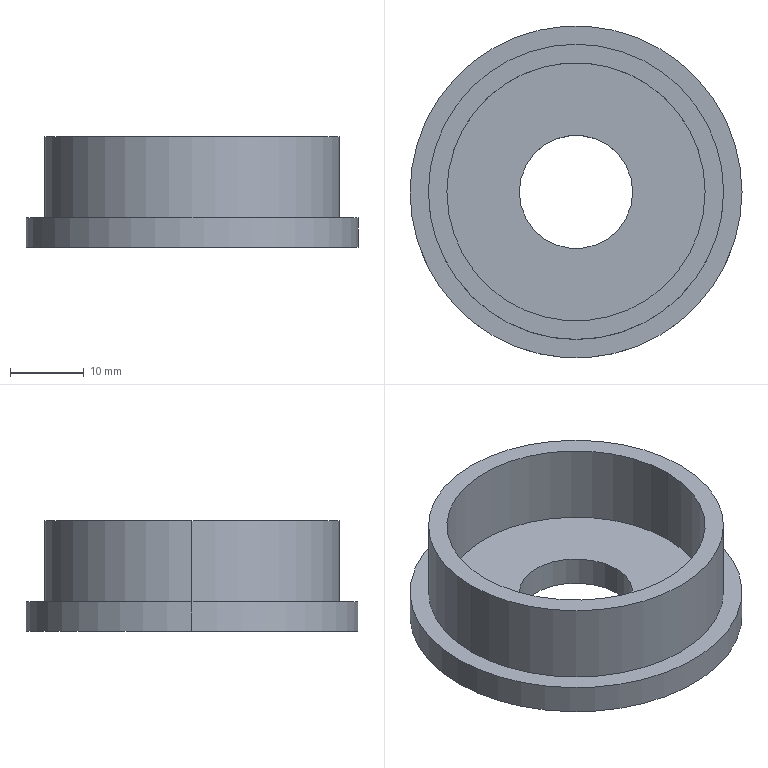Part | SolidWorks | features ICE 2, Extrusion 1 | 1 solid | 12 faces | box 45 x 45 x 15 mm | volume 8861 mm3 | cylinder 8 | plane 4 | commonest cylinder face diameters 15.357 x2 35 x2 40 x2 45 x2
STEP:
#1=CARTESIAN_POINT('',(-7.679,0.,-2.));
#2=VERTEX_POINT('',#1);
#3=CARTESIAN_POINT('',(7.679,0.,-2.));
#4=VERTEX_POINT('',#3);
#5=CARTESIAN_POINT('',(0.,0.,-2.));
#6=DIRECTION('',(0.,0.,1.));
#7=DIRECTION('',(1.,0.,0.));
#8=AXIS2_PLACEMENT_3D('',#5,#6,#7);
#9=CIRCLE('',#8,7.679);
#10=EDGE_CURVE('',#2,#4,#9,.T.);
#11=ORIENTED_EDGE('',*,*,#10,.F.);
#12=CARTESIAN_POINT('',(-7.679,0.,2.));
#13=VERTEX_POINT('',#12);
#14=CARTESIAN_POINT('',(-7.679,0.,-19.));
#15=DIRECTION('',(0.,0.,1.));
#16=VECTOR('',#15,1000.);
#17=LINE('',#14,#16);
#18=EDGE_CURVE('',#2,#13,#17,.T.);
#19=ORIENTED_EDGE('',*,*,#18,.T.);
#20=CARTESIAN_POINT('',(7.679,0.,2.));
#21=VERTEX_POINT('',#20);
#22=CARTESIAN_POINT('',(0.,0.,2.));
#23=DIRECTION('',(0.,0.,1.));
#24=DIRECTION('',(1.,0.,0.));
#25=AXIS2_PLACEMENT_3D('',#22,#23,#24);
#26=CIRCLE('',#25,7.679);
#27=EDGE_CURVE('',#13,#21,#26,.T.);
#28=ORIENTED_EDGE('',*,*,#27,.T.);
#29=CARTESIAN_POINT('',(7.679,0.,-19.));
#30=DIRECTION('',(0.,0.,1.));
#31=VECTOR('',#30,1000.);
#32=LINE('',#29,#31);
#33=EDGE_CURVE('',#4,#21,#32,.T.);
#34=ORIENTED_EDGE('',*,*,#33,.F.);
#35=EDGE_LOOP('',(#11,#19,#28,#34));
#36=FACE_OUTER_BOUND('',#35,.T.);
#37=CARTESIAN_POINT('',(0.,0.,-19.));
#38=DIRECTION('',(0.,0.,1.));
#39=DIRECTION('',(1.,0.,0.));
#40=AXIS2_PLACEMENT_3D('',#37,#38,#39);
#41=CYLINDRICAL_SURFACE('',#40,7.679);
#42=ADVANCED_FACE('',(#36),#41,.F.);
#43=CARTESIAN_POINT('',(-17.5,0.,13.));
#44=VERTEX_POINT('',#43);
#45=CARTESIAN_POINT('',(17.5,0.,13.));
#46=VERTEX_POINT('',#45);
#47=CARTESIAN_POINT('',(0.,0.,13.));
#48=DIRECTION('',(0.,0.,1.));
#49=DIRECTION('',(1.,0.,0.));
#50=AXIS2_PLACEMENT_3D('',#47,#48,#49);
#51=CIRCLE('',#50,17.5);
#52=EDGE_CURVE('',#44,#46,#51,.T.);
#53=ORIENTED_EDGE('',*,*,#52,.T.);
#54=CARTESIAN_POINT('',(17.5,0.,2.));
#55=VERTEX_POINT('',#54);
#56=CARTESIAN_POINT('',(17.5,0.,13.));
#57=DIRECTION('',(0.,0.,-1.));
#58=VECTOR('',#57,1000.);
#59=LINE('',#56,#58);
#60=EDGE_CURVE('',#46,#55,#59,.T.);
#61=ORIENTED_EDGE('',*,*,#60,.T.);
#62=CARTESIAN_POINT('',(-17.5,0.,2.));
#63=VERTEX_POINT('',#62);
#64=CARTESIAN_POINT('',(0.,0.,2.));
#65=DIRECTION('',(0.,0.,-1.));
#66=DIRECTION('',(1.,0.,0.));
#67=AXIS2_PLACEMENT_3D('',#64,#65,#66);
#68=CIRCLE('',#67,17.5);
#69=EDGE_CURVE('',#55,#63,#68,.T.);
#70=ORIENTED_EDGE('',*,*,#69,.T.);
#71=CARTESIAN_POINT('',(-17.5,0.,13.));
#72=DIRECTION('',(0.,0.,-1.));
#73=VECTOR('',#72,1000.);
#74=LINE('',#71,#73);
#75=EDGE_CURVE('',#44,#63,#74,.T.);
#76=ORIENTED_EDGE('',*,*,#75,.F.);
#77=EDGE_LOOP('',(#53,#61,#70,#76));
#78=FACE_OUTER_BOUND('',#77,.T.);
#79=CARTESIAN_POINT('',(0.,0.,13.));
#80=DIRECTION('',(0.,0.,-1.));
#81=DIRECTION('',(-1.,0.,0.));
#82=AXIS2_PLACEMENT_3D('',#79,#80,#81);
#83=CYLINDRICAL_SURFACE('',#82,17.5);
#84=ADVANCED_FACE('',(#78),#83,.F.);
#85=CARTESIAN_POINT('',(20.,0.,13.));
#86=VERTEX_POINT('',#85);
#87=CARTESIAN_POINT('',(-20.,0.,13.));
#88=VERTEX_POINT('',#87);
#89=CARTESIAN_POINT('',(0.,0.,13.));
#90=DIRECTION('',(0.,0.,1.));
#91=DIRECTION('',(1.,0.,0.));
#92=AXIS2_PLACEMENT_3D('',#89,#90,#91);
#93=CIRCLE('',#92,20.);
#94=EDGE_CURVE('',#86,#88,#93,.T.);
#95=ORIENTED_EDGE('',*,*,#94,.F.);
#96=CARTESIAN_POINT('',(20.,0.,2.));
#97=VERTEX_POINT('',#96);
#98=CARTESIAN_POINT('',(20.,0.,13.));
#99=DIRECTION('',(0.,0.,-1.));
#100=VECTOR('',#99,1000.);
#101=LINE('',#98,#100);
#102=EDGE_CURVE('',#86,#97,#101,.T.);
#103=ORIENTED_EDGE('',*,*,#102,.T.);
#104=CARTESIAN_POINT('',(-20.,0.,2.));
#105=VERTEX_POINT('',#104);
#106=CARTESIAN_POINT('',(0.,0.,2.));
#107=DIRECTION('',(0.,0.,1.));
#108=DIRECTION('',(1.,0.,0.));
#109=AXIS2_PLACEMENT_3D('',#106,#107,#108);
#110=CIRCLE('',#109,20.);
#111=EDGE_CURVE('',#97,#105,#110,.T.);
#112=ORIENTED_EDGE('',*,*,#111,.T.);
#113=CARTESIAN_POINT('',(-20.,0.,13.));
#114=DIRECTION('',(0.,0.,-1.));
#115=VECTOR('',#114,1000.);
#116=LINE('',#113,#115);
#117=EDGE_CURVE('',#88,#105,#116,.T.);
#118=ORIENTED_EDGE('',*,*,#117,.F.);
#119=EDGE_LOOP('',(#95,#103,#112,#118));
#120=FACE_OUTER_BOUND('',#119,.T.);
#121=CARTESIAN_POINT('',(0.,0.,13.));
#122=DIRECTION('',(0.,0.,-1.));
#123=DIRECTION('',(-1.,0.,0.));
#124=AXIS2_PLACEMENT_3D('',#121,#122,#123);
#125=CYLINDRICAL_SURFACE('',#124,20.);
#126=ADVANCED_FACE('',(#120),#125,.T.);
#127=CARTESIAN_POINT('',(22.5,0.,2.));
#128=VERTEX_POINT('',#127);
#129=CARTESIAN_POINT('',(-22.5,0.,2.));
#130=VERTEX_POINT('',#129);
#131=CARTESIAN_POINT('',(0.,0.,2.));
#132=DIRECTION('',(0.,0.,1.));
#133=DIRECTION('',(1.,0.,0.));
#134=AXIS2_PLACEMENT_3D('',#131,#132,#133);
#135=CIRCLE('',#134,22.5);
#136=EDGE_CURVE('',#128,#130,#135,.T.);
#137=ORIENTED_EDGE('',*,*,#136,.F.);
#138=CARTESIAN_POINT('',(22.5,0.,-2.));
#139=VERTEX_POINT('',#138);
#140=CARTESIAN_POINT('',(22.5,0.,2.));
#141=DIRECTION('',(0.,0.,-1.));
#142=VECTOR('',#141,1000.);
#143=LINE('',#140,#142);
#144=EDGE_CURVE('',#128,#139,#143,.T.);
#145=ORIENTED_EDGE('',*,*,#144,.T.);
#146=CARTESIAN_POINT('',(-22.5,0.,-2.));
#147=VERTEX_POINT('',#146);
#148=CARTESIAN_POINT('',(0.,0.,-2.));
#149=DIRECTION('',(0.,0.,1.));
#150=DIRECTION('',(1.,0.,0.));
#151=AXIS2_PLACEMENT_3D('',#148,#149,#150);
#152=CIRCLE('',#151,22.5);
#153=EDGE_CURVE('',#139,#147,#152,.T.);
#154=ORIENTED_EDGE('',*,*,#153,.T.);
#155=CARTESIAN_POINT('',(-22.5,0.,2.));
#156=DIRECTION('',(0.,0.,-1.));
#157=VECTOR('',#156,1000.);
#158=LINE('',#155,#157);
#159=EDGE_CURVE('',#130,#147,#158,.T.);
#160=ORIENTED_EDGE('',*,*,#159,.F.);
#161=EDGE_LOOP('',(#137,#145,#154,#160));
#162=FACE_OUTER_BOUND('',#161,.T.);
#163=CARTESIAN_POINT('',(0.,0.,2.));
#164=DIRECTION('',(0.,0.,-1.));
#165=DIRECTION('',(-1.,0.,0.));
#166=AXIS2_PLACEMENT_3D('',#163,#164,#165);
#167=CYLINDRICAL_SURFACE('',#166,22.5);
#168=ADVANCED_FACE('',(#162),#167,.T.);
#169=ORIENTED_EDGE('',*,*,#144,.F.);
#170=CARTESIAN_POINT('',(0.,0.,2.));
#171=DIRECTION('',(0.,0.,1.));
#172=DIRECTION('',(1.,0.,0.));
#173=AXIS2_PLACEMENT_3D('',#170,#171,#172);
#174=CIRCLE('',#173,22.5);
#175=EDGE_CURVE('',#130,#128,#174,.T.);
#176=ORIENTED_EDGE('',*,*,#175,.F.);
#177=ORIENTED_EDGE('',*,*,#159,.T.);
#178=CARTESIAN_POINT('',(0.,0.,-2.));
#179=DIRECTION('',(0.,0.,1.));
#180=DIRECTION('',(1.,0.,0.));
#181=AXIS2_PLACEMENT_3D('',#178,#179,#180);
#182=CIRCLE('',#181,22.5);
#183=EDGE_CURVE('',#147,#139,#182,.T.);
#184=ORIENTED_EDGE('',*,*,#183,.T.);
#185=EDGE_LOOP('',(#169,#176,#177,#184));
#186=FACE_OUTER_BOUND('',#185,.T.);
#187=CARTESIAN_POINT('',(0.,0.,2.));
#188=DIRECTION('',(0.,0.,-1.));
#189=DIRECTION('',(-1.,0.,0.));
#190=AXIS2_PLACEMENT_3D('',#187,#188,#189);
#191=CYLINDRICAL_SURFACE('',#190,22.5);
#192=ADVANCED_FACE('',(#186),#191,.T.);
#193=CARTESIAN_POINT('',(0.,0.,2.));
#194=DIRECTION('',(0.,0.,1.));
#195=DIRECTION('',(1.,0.,0.));
#196=AXIS2_PLACEMENT_3D('',#193,#194,#195);
#197=CIRCLE('',#196,20.);
#198=EDGE_CURVE('',#105,#97,#197,.T.);
#199=ORIENTED_EDGE('',*,*,#198,.F.);
#200=ORIENTED_EDGE('',*,*,#111,.F.);
#201=EDGE_LOOP('',(#199,#200));
#202=FACE_BOUND('',#201,.T.);
#203=ORIENTED_EDGE('',*,*,#175,.T.);
#204=ORIENTED_EDGE('',*,*,#136,.T.);
#205=EDGE_LOOP('',(#203,#204));
#206=FACE_OUTER_BOUND('',#205,.T.);
#207=CARTESIAN_POINT('',(0.,0.,2.));
#208=DIRECTION('',(0.,0.,1.));
#209=DIRECTION('',(1.,0.,0.));
#210=AXIS2_PLACEMENT_3D('',#207,#208,#209);
#211=PLANE('',#210);
#212=ADVANCED_FACE('',(#202,#206),#211,.T.);
#213=CARTESIAN_POINT('',(0.,0.,-2.));
#214=DIRECTION('',(0.,0.,1.));
#215=DIRECTION('',(1.,0.,0.));
#216=AXIS2_PLACEMENT_3D('',#213,#214,#215);
#217=CIRCLE('',#216,7.679);
#218=EDGE_CURVE('',#4,#2,#217,.T.);
#219=ORIENTED_EDGE('',*,*,#218,.T.);
#220=ORIENTED_EDGE('',*,*,#10,.T.);
#221=EDGE_LOOP('',(#219,#220));
#222=FACE_BOUND('',#221,.T.);
#223=ORIENTED_EDGE('',*,*,#183,.F.);
#224=ORIENTED_EDGE('',*,*,#153,.F.);
#225=EDGE_LOOP('',(#223,#224));
#226=FACE_OUTER_BOUND('',#225,.T.);
#227=CARTESIAN_POINT('',(0.,0.,-2.));
#228=DIRECTION('',(0.,0.,1.));
#229=DIRECTION('',(1.,0.,0.));
#230=AXIS2_PLACEMENT_3D('',#227,#228,#229);
#231=PLANE('',#230);
#232=ADVANCED_FACE('',(#222,#226),#231,.F.);
#233=CARTESIAN_POINT('',(0.,0.,13.));
#234=DIRECTION('',(0.,0.,1.));
#235=DIRECTION('',(1.,0.,0.));
#236=AXIS2_PLACEMENT_3D('',#233,#234,#235);
#237=CIRCLE('',#236,20.);
#238=EDGE_CURVE('',#88,#86,#237,.T.);
#239=ORIENTED_EDGE('',*,*,#238,.T.);
#240=ORIENTED_EDGE('',*,*,#94,.T.);
#241=EDGE_LOOP('',(#239,#240));
#242=FACE_OUTER_BOUND('',#241,.T.);
#243=ORIENTED_EDGE('',*,*,#52,.F.);
#244=CARTESIAN_POINT('',(0.,0.,13.));
#245=DIRECTION('',(0.,0.,1.));
#246=DIRECTION('',(1.,0.,0.));
#247=AXIS2_PLACEMENT_3D('',#244,#245,#246);
#248=CIRCLE('',#247,17.5);
#249=EDGE_CURVE('',#46,#44,#248,.T.);
#250=ORIENTED_EDGE('',*,*,#249,.F.);
#251=EDGE_LOOP('',(#243,#250));
#252=FACE_BOUND('',#251,.T.);
#253=CARTESIAN_POINT('',(0.,0.,13.));
#254=DIRECTION('',(0.,0.,1.));
#255=DIRECTION('',(1.,0.,0.));
#256=AXIS2_PLACEMENT_3D('',#253,#254,#255);
#257=PLANE('',#256);
#258=ADVANCED_FACE('',(#242,#252),#257,.T.);
#259=ORIENTED_EDGE('',*,*,#102,.F.);
#260=ORIENTED_EDGE('',*,*,#238,.F.);
#261=ORIENTED_EDGE('',*,*,#117,.T.);
#262=ORIENTED_EDGE('',*,*,#198,.T.);
#263=EDGE_LOOP('',(#259,#260,#261,#262));
#264=FACE_OUTER_BOUND('',#263,.T.);
#265=CARTESIAN_POINT('',(0.,0.,13.));
#266=DIRECTION('',(0.,0.,-1.));
#267=DIRECTION('',(-1.,0.,0.));
#268=AXIS2_PLACEMENT_3D('',#265,#266,#267);
#269=CYLINDRICAL_SURFACE('',#268,20.);
#270=ADVANCED_FACE('',(#264),#269,.T.);
#271=ORIENTED_EDGE('',*,*,#60,.F.);
#272=ORIENTED_EDGE('',*,*,#249,.T.);
#273=ORIENTED_EDGE('',*,*,#75,.T.);
#274=CARTESIAN_POINT('',(0.,0.,2.));
#275=DIRECTION('',(0.,0.,-1.));
#276=DIRECTION('',(1.,0.,0.));
#277=AXIS2_PLACEMENT_3D('',#274,#275,#276);
#278=CIRCLE('',#277,17.5);
#279=EDGE_CURVE('',#63,#55,#278,.T.);
#280=ORIENTED_EDGE('',*,*,#279,.T.);
#281=EDGE_LOOP('',(#271,#272,#273,#280));
#282=FACE_OUTER_BOUND('',#281,.T.);
#283=CARTESIAN_POINT('',(0.,0.,13.));
#284=DIRECTION('',(0.,0.,-1.));
#285=DIRECTION('',(-1.,0.,0.));
#286=AXIS2_PLACEMENT_3D('',#283,#284,#285);
#287=CYLINDRICAL_SURFACE('',#286,17.5);
#288=ADVANCED_FACE('',(#282),#287,.F.);
#289=CARTESIAN_POINT('',(0.,0.,2.));
#290=DIRECTION('',(0.,0.,1.));
#291=DIRECTION('',(1.,0.,0.));
#292=AXIS2_PLACEMENT_3D('',#289,#290,#291);
#293=CIRCLE('',#292,7.679);
#294=EDGE_CURVE('',#21,#13,#293,.T.);
#295=ORIENTED_EDGE('',*,*,#294,.F.);
#296=ORIENTED_EDGE('',*,*,#27,.F.);
#297=EDGE_LOOP('',(#295,#296));
#298=FACE_BOUND('',#297,.T.);
#299=ORIENTED_EDGE('',*,*,#279,.F.);
#300=ORIENTED_EDGE('',*,*,#69,.F.);
#301=EDGE_LOOP('',(#299,#300));
#302=FACE_OUTER_BOUND('',#301,.T.);
#303=CARTESIAN_POINT('',(0.,0.,2.));
#304=DIRECTION('',(0.,0.,1.));
#305=DIRECTION('',(1.,0.,0.));
#306=AXIS2_PLACEMENT_3D('',#303,#304,#305);
#307=PLANE('',#306);
#308=ADVANCED_FACE('',(#298,#302),#307,.T.);
#309=ORIENTED_EDGE('',*,*,#18,.F.);
#310=ORIENTED_EDGE('',*,*,#218,.F.);
#311=ORIENTED_EDGE('',*,*,#33,.T.);
#312=ORIENTED_EDGE('',*,*,#294,.T.);
#313=EDGE_LOOP('',(#309,#310,#311,#312));
#314=FACE_OUTER_BOUND('',#313,.T.);
#315=CARTESIAN_POINT('',(0.,0.,-19.));
#316=DIRECTION('',(0.,0.,1.));
#317=DIRECTION('',(1.,0.,0.));
#318=AXIS2_PLACEMENT_3D('',#315,#316,#317);
#319=CYLINDRICAL_SURFACE('',#318,7.679);
#320=ADVANCED_FACE('',(#314),#319,.F.);
#321=CLOSED_SHELL('',(#42,#84,#126,#168,#192,#212,#232,#258,#270,#288,#308,#320));
#322=MANIFOLD_SOLID_BREP('',#321);
#323=CARTESIAN_POINT('',(0.,0.,0.));
#324=DIRECTION('',(0.,0.,1.));
#325=DIRECTION('',(1.,0.,0.));
#326=AXIS2_PLACEMENT_3D('',#323,#324,#325);
#327=(LENGTH_UNIT()NAMED_UNIT(*)SI_UNIT(.MILLI.,.METRE.));
#328=UNCERTAINTY_MEASURE_WITH_UNIT(LENGTH_MEASURE(0.00001),#327,'','');
#329=(NAMED_UNIT(*)PLANE_ANGLE_UNIT()SI_UNIT($,.RADIAN.));
#330=(NAMED_UNIT(*)SI_UNIT($,.STERADIAN.)SOLID_ANGLE_UNIT());
#331=(GEOMETRIC_REPRESENTATION_CONTEXT(3)GLOBAL_UNCERTAINTY_ASSIGNED_CONTEXT((#328))GLOBAL_UNIT_ASSIGNED_CONTEXT((#327,#329,#330))REPRESENTATION_CONTEXT('',''));
#332=ADVANCED_BREP_SHAPE_REPRESENTATION('',(#322,#326),#331);